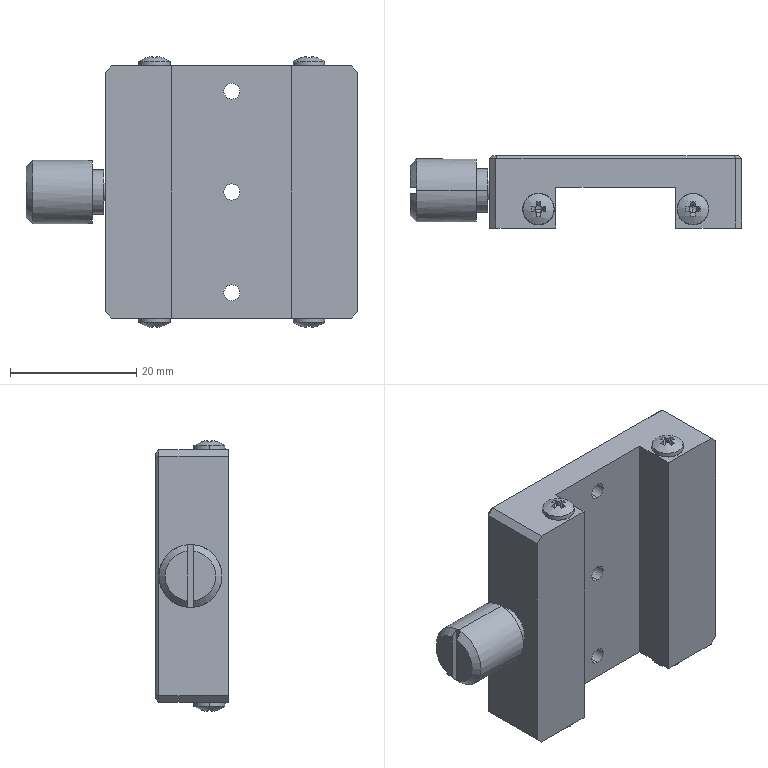Part | STEP file | Guide wheel mechanism revised.sldasm-Part-380 | 1 solid | 195 faces | box 52.6 x 11.5 x 42.9 mm | volume 14076 mm3 | plane 106 | cone 51 | cylinder 34 | sphere 4 | commonest cylinder face diameters 2.55 x18 5 x8 3 x4 7 x2 10 x2